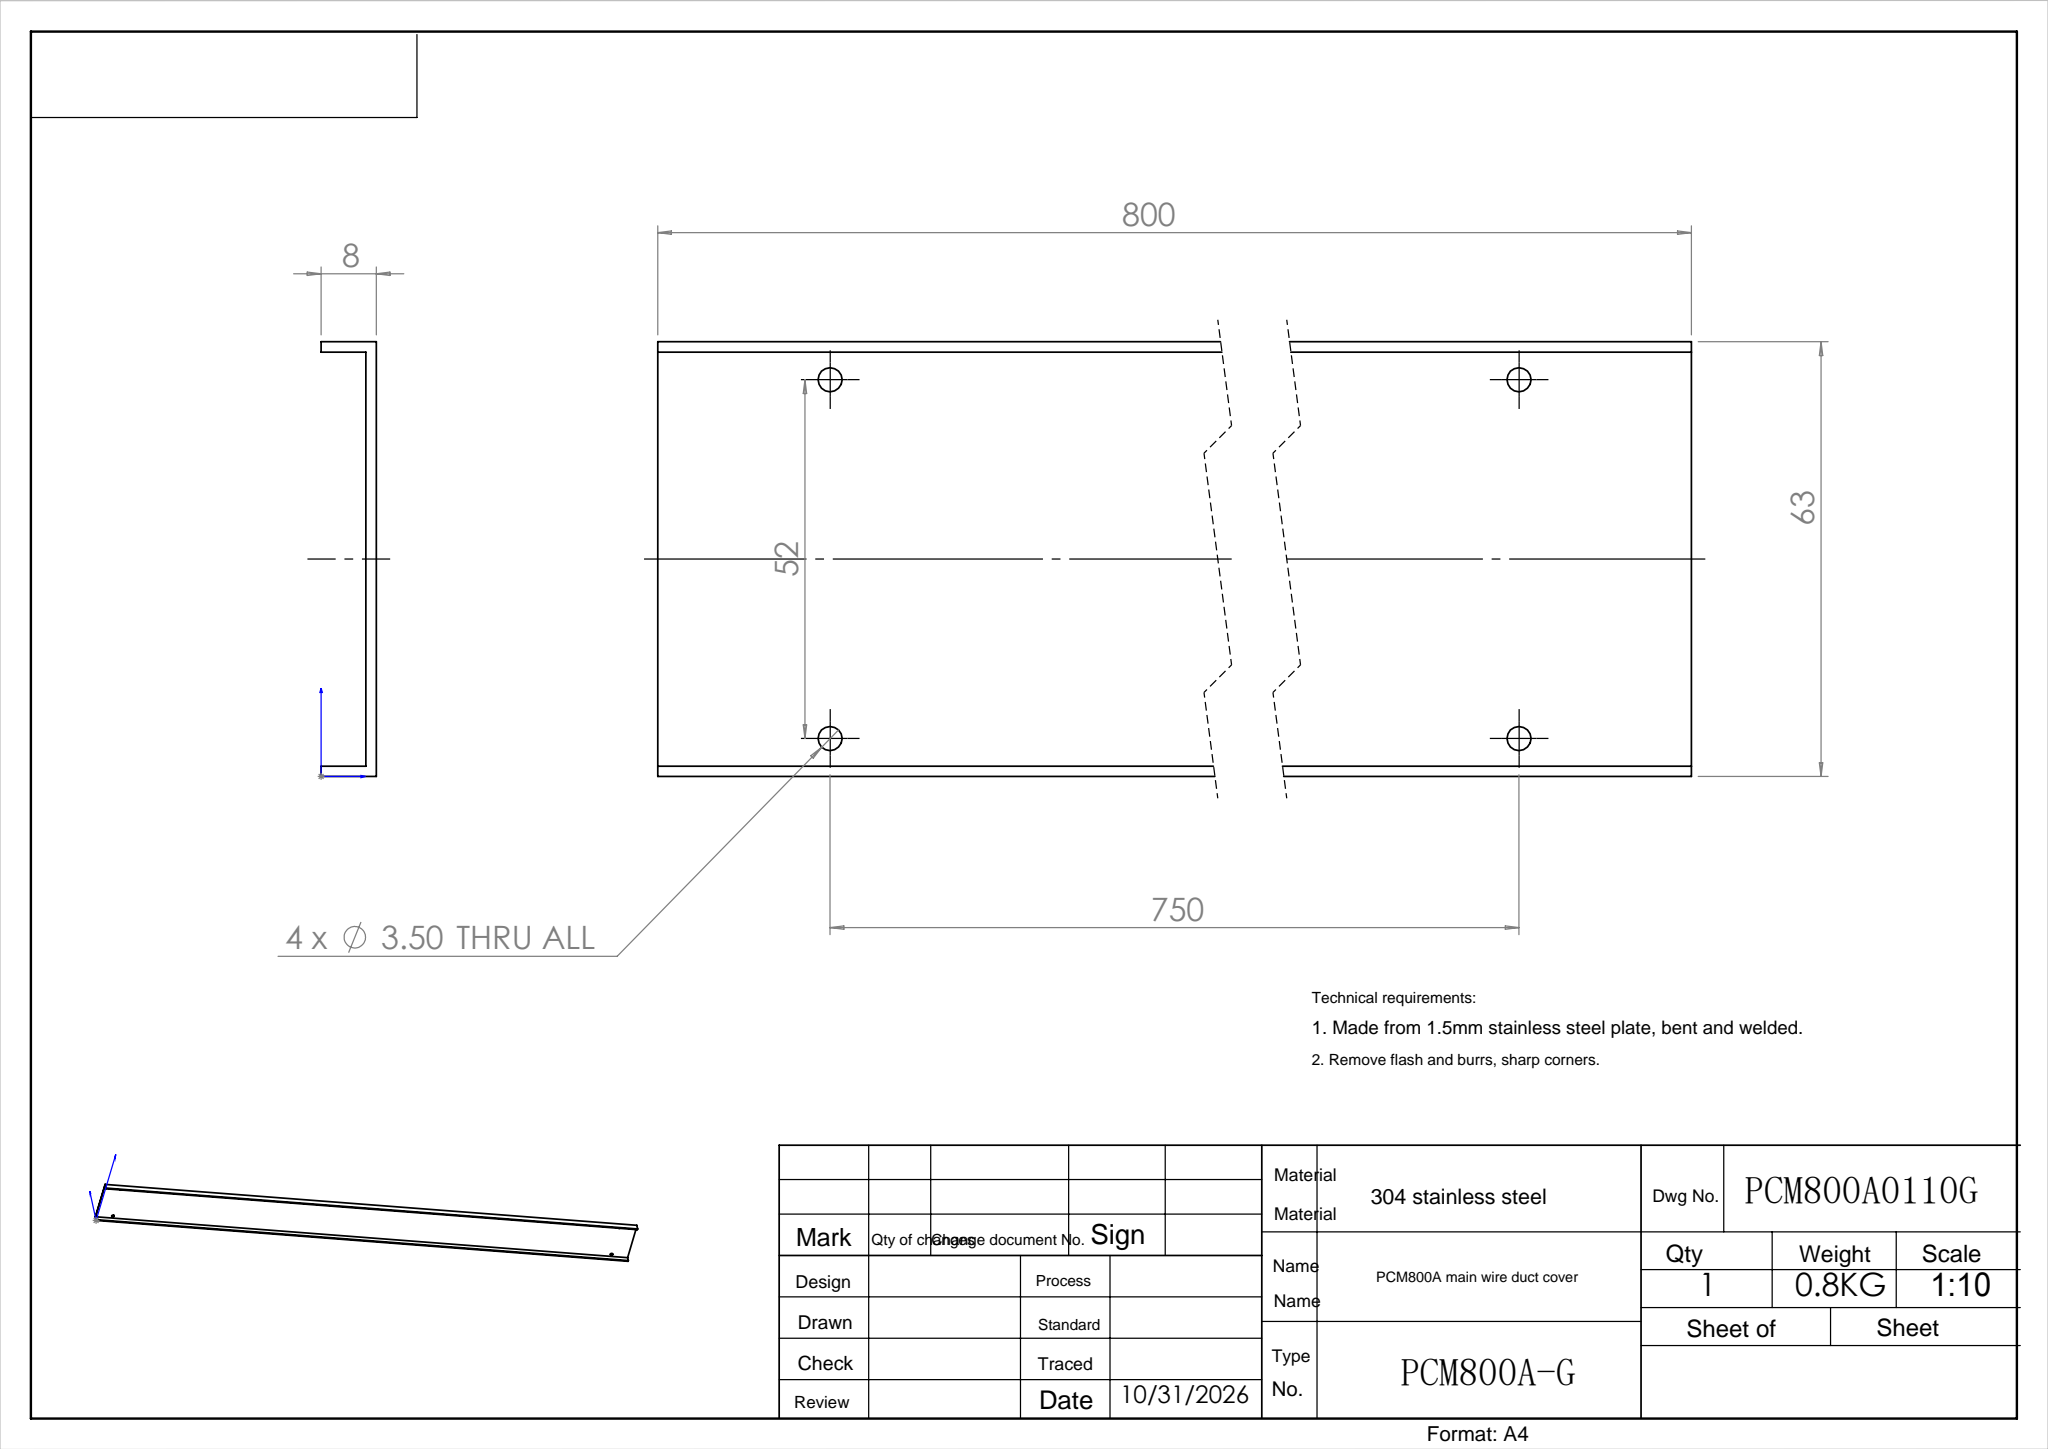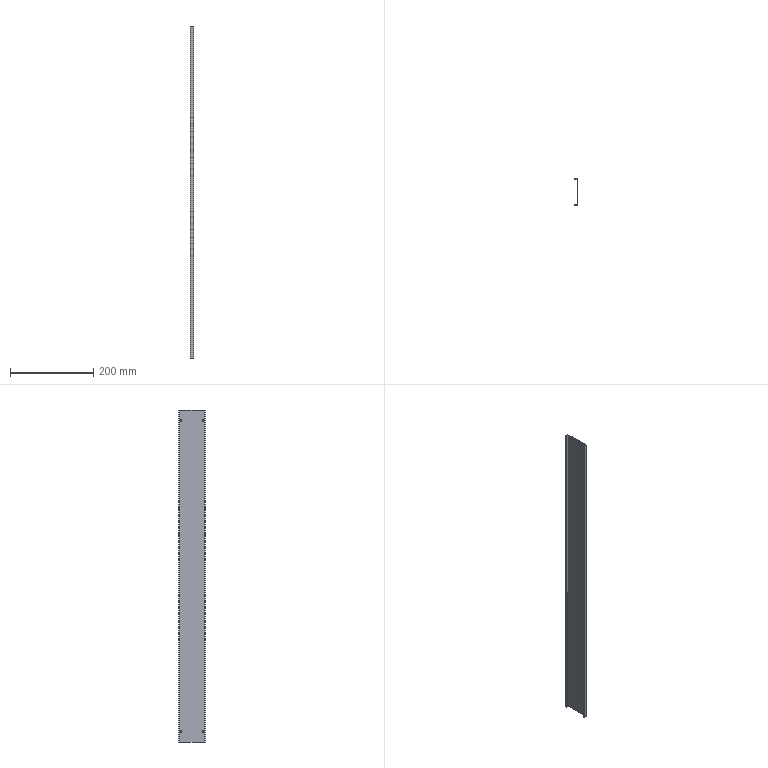Part | SolidWorks | features ExtruThin 1, HoleWzd 1, MirrorPattern 1 | 1 solid | 18 faces | box 8 x 63 x 800 mm | volume 91142 mm3 | plane 10 | cylinder 8 | commonest cylinder face diameters 3.5 x8
STEP:
#1=CARTESIAN_POINT('',(6.5,5.5,773.25));
#2=VERTEX_POINT('',#1);
#3=CARTESIAN_POINT('',(6.5,5.5,776.75));
#4=VERTEX_POINT('',#3);
#5=CARTESIAN_POINT('',(6.5,5.5,775.));
#6=DIRECTION('',(-1.,0.,0.));
#7=DIRECTION('',(0.,0.,1.));
#8=AXIS2_PLACEMENT_3D('',#5,#6,#7);
#9=CIRCLE('',#8,1.75);
#10=EDGE_CURVE('',#2,#4,#9,.T.);
#11=ORIENTED_EDGE('',*,*,#10,.T.);
#12=CARTESIAN_POINT('',(8.,5.5,776.75));
#13=VERTEX_POINT('',#12);
#14=CARTESIAN_POINT('',(8.,5.5,776.75));
#15=DIRECTION('',(1.,0.,0.));
#16=VECTOR('',#15,1000.);
#17=LINE('',#14,#16);
#18=EDGE_CURVE('',#4,#13,#17,.T.);
#19=ORIENTED_EDGE('',*,*,#18,.T.);
#20=CARTESIAN_POINT('',(8.,5.5,773.25));
#21=VERTEX_POINT('',#20);
#22=CARTESIAN_POINT('',(8.,5.5,775.));
#23=DIRECTION('',(1.,0.,0.));
#24=DIRECTION('',(0.,0.,-1.));
#25=AXIS2_PLACEMENT_3D('',#22,#23,#24);
#26=CIRCLE('',#25,1.75);
#27=EDGE_CURVE('',#13,#21,#26,.T.);
#28=ORIENTED_EDGE('',*,*,#27,.T.);
#29=CARTESIAN_POINT('',(8.,5.5,773.25));
#30=DIRECTION('',(1.,0.,0.));
#31=VECTOR('',#30,1000.);
#32=LINE('',#29,#31);
#33=EDGE_CURVE('',#2,#21,#32,.T.);
#34=ORIENTED_EDGE('',*,*,#33,.F.);
#35=EDGE_LOOP('',(#11,#19,#28,#34));
#36=FACE_OUTER_BOUND('',#35,.T.);
#37=CARTESIAN_POINT('',(8.,5.5,775.));
#38=DIRECTION('',(1.,0.,0.));
#39=DIRECTION('',(0.,0.,-1.));
#40=AXIS2_PLACEMENT_3D('',#37,#38,#39);
#41=CYLINDRICAL_SURFACE('',#40,1.75);
#42=ADVANCED_FACE('',(#36),#41,.F.);
#43=CARTESIAN_POINT('',(6.5,5.5,23.25));
#44=VERTEX_POINT('',#43);
#45=CARTESIAN_POINT('',(6.5,5.5,26.75));
#46=VERTEX_POINT('',#45);
#47=CARTESIAN_POINT('',(6.5,5.5,25.));
#48=DIRECTION('',(-1.,0.,0.));
#49=DIRECTION('',(0.,0.,1.));
#50=AXIS2_PLACEMENT_3D('',#47,#48,#49);
#51=CIRCLE('',#50,1.75);
#52=EDGE_CURVE('',#44,#46,#51,.T.);
#53=ORIENTED_EDGE('',*,*,#52,.T.);
#54=CARTESIAN_POINT('',(8.,5.5,26.75));
#55=VERTEX_POINT('',#54);
#56=CARTESIAN_POINT('',(8.,5.5,26.75));
#57=DIRECTION('',(1.,0.,0.));
#58=VECTOR('',#57,1000.);
#59=LINE('',#56,#58);
#60=EDGE_CURVE('',#46,#55,#59,.T.);
#61=ORIENTED_EDGE('',*,*,#60,.T.);
#62=CARTESIAN_POINT('',(8.,5.5,23.25));
#63=VERTEX_POINT('',#62);
#64=CARTESIAN_POINT('',(8.,5.5,25.));
#65=DIRECTION('',(1.,0.,0.));
#66=DIRECTION('',(0.,0.,-1.));
#67=AXIS2_PLACEMENT_3D('',#64,#65,#66);
#68=CIRCLE('',#67,1.75);
#69=EDGE_CURVE('',#55,#63,#68,.T.);
#70=ORIENTED_EDGE('',*,*,#69,.T.);
#71=CARTESIAN_POINT('',(8.,5.5,23.25));
#72=DIRECTION('',(1.,0.,0.));
#73=VECTOR('',#72,1000.);
#74=LINE('',#71,#73);
#75=EDGE_CURVE('',#44,#63,#74,.T.);
#76=ORIENTED_EDGE('',*,*,#75,.F.);
#77=EDGE_LOOP('',(#53,#61,#70,#76));
#78=FACE_OUTER_BOUND('',#77,.T.);
#79=CARTESIAN_POINT('',(8.,5.5,25.));
#80=DIRECTION('',(1.,0.,0.));
#81=DIRECTION('',(0.,0.,-1.));
#82=AXIS2_PLACEMENT_3D('',#79,#80,#81);
#83=CYLINDRICAL_SURFACE('',#82,1.75);
#84=ADVANCED_FACE('',(#78),#83,.F.);
#85=CARTESIAN_POINT('',(6.5,57.5,773.25));
#86=VERTEX_POINT('',#85);
#87=CARTESIAN_POINT('',(6.5,57.5,776.75));
#88=VERTEX_POINT('',#87);
#89=CARTESIAN_POINT('',(6.5,57.5,775.));
#90=DIRECTION('',(-1.,0.,0.));
#91=DIRECTION('',(0.,0.,1.));
#92=AXIS2_PLACEMENT_3D('',#89,#90,#91);
#93=CIRCLE('',#92,1.75);
#94=EDGE_CURVE('',#86,#88,#93,.T.);
#95=ORIENTED_EDGE('',*,*,#94,.T.);
#96=CARTESIAN_POINT('',(8.,57.5,776.75));
#97=VERTEX_POINT('',#96);
#98=CARTESIAN_POINT('',(8.,57.5,776.75));
#99=DIRECTION('',(1.,0.,0.));
#100=VECTOR('',#99,1000.);
#101=LINE('',#98,#100);
#102=EDGE_CURVE('',#88,#97,#101,.T.);
#103=ORIENTED_EDGE('',*,*,#102,.T.);
#104=CARTESIAN_POINT('',(8.,57.5,773.25));
#105=VERTEX_POINT('',#104);
#106=CARTESIAN_POINT('',(8.,57.5,775.));
#107=DIRECTION('',(1.,0.,0.));
#108=DIRECTION('',(0.,0.,-1.));
#109=AXIS2_PLACEMENT_3D('',#106,#107,#108);
#110=CIRCLE('',#109,1.75);
#111=EDGE_CURVE('',#97,#105,#110,.T.);
#112=ORIENTED_EDGE('',*,*,#111,.T.);
#113=CARTESIAN_POINT('',(8.,57.5,773.25));
#114=DIRECTION('',(1.,0.,0.));
#115=VECTOR('',#114,1000.);
#116=LINE('',#113,#115);
#117=EDGE_CURVE('',#86,#105,#116,.T.);
#118=ORIENTED_EDGE('',*,*,#117,.F.);
#119=EDGE_LOOP('',(#95,#103,#112,#118));
#120=FACE_OUTER_BOUND('',#119,.T.);
#121=CARTESIAN_POINT('',(8.,57.5,775.));
#122=DIRECTION('',(1.,0.,0.));
#123=DIRECTION('',(0.,0.,-1.));
#124=AXIS2_PLACEMENT_3D('',#121,#122,#123);
#125=CYLINDRICAL_SURFACE('',#124,1.75);
#126=ADVANCED_FACE('',(#120),#125,.F.);
#127=CARTESIAN_POINT('',(6.5,57.5,23.25));
#128=VERTEX_POINT('',#127);
#129=CARTESIAN_POINT('',(6.5,57.5,26.75));
#130=VERTEX_POINT('',#129);
#131=CARTESIAN_POINT('',(6.5,57.5,25.));
#132=DIRECTION('',(-1.,0.,0.));
#133=DIRECTION('',(0.,0.,1.));
#134=AXIS2_PLACEMENT_3D('',#131,#132,#133);
#135=CIRCLE('',#134,1.75);
#136=EDGE_CURVE('',#128,#130,#135,.T.);
#137=ORIENTED_EDGE('',*,*,#136,.T.);
#138=CARTESIAN_POINT('',(8.,57.5,26.75));
#139=VERTEX_POINT('',#138);
#140=CARTESIAN_POINT('',(8.,57.5,26.75));
#141=DIRECTION('',(1.,0.,0.));
#142=VECTOR('',#141,1000.);
#143=LINE('',#140,#142);
#144=EDGE_CURVE('',#130,#139,#143,.T.);
#145=ORIENTED_EDGE('',*,*,#144,.T.);
#146=CARTESIAN_POINT('',(8.,57.5,23.25));
#147=VERTEX_POINT('',#146);
#148=CARTESIAN_POINT('',(8.,57.5,25.));
#149=DIRECTION('',(1.,0.,0.));
#150=DIRECTION('',(0.,0.,-1.));
#151=AXIS2_PLACEMENT_3D('',#148,#149,#150);
#152=CIRCLE('',#151,1.75);
#153=EDGE_CURVE('',#139,#147,#152,.T.);
#154=ORIENTED_EDGE('',*,*,#153,.T.);
#155=CARTESIAN_POINT('',(8.,57.5,23.25));
#156=DIRECTION('',(1.,0.,0.));
#157=VECTOR('',#156,1000.);
#158=LINE('',#155,#157);
#159=EDGE_CURVE('',#128,#147,#158,.T.);
#160=ORIENTED_EDGE('',*,*,#159,.F.);
#161=EDGE_LOOP('',(#137,#145,#154,#160));
#162=FACE_OUTER_BOUND('',#161,.T.);
#163=CARTESIAN_POINT('',(8.,57.5,25.));
#164=DIRECTION('',(1.,0.,0.));
#165=DIRECTION('',(0.,0.,-1.));
#166=AXIS2_PLACEMENT_3D('',#163,#164,#165);
#167=CYLINDRICAL_SURFACE('',#166,1.75);
#168=ADVANCED_FACE('',(#162),#167,.F.);
#169=CARTESIAN_POINT('',(8.,63.,0.));
#170=VERTEX_POINT('',#169);
#171=CARTESIAN_POINT('',(0.,63.,0.));
#172=VERTEX_POINT('',#171);
#173=CARTESIAN_POINT('',(8.,63.,0.));
#174=DIRECTION('',(-1.,0.,0.));
#175=VECTOR('',#174,1000.);
#176=LINE('',#173,#175);
#177=EDGE_CURVE('',#170,#172,#176,.T.);
#178=ORIENTED_EDGE('',*,*,#177,.T.);
#179=CARTESIAN_POINT('',(0.,63.,800.));
#180=VERTEX_POINT('',#179);
#181=CARTESIAN_POINT('',(0.,63.,800.));
#182=DIRECTION('',(0.,0.,-1.));
#183=VECTOR('',#182,1000.);
#184=LINE('',#181,#183);
#185=EDGE_CURVE('',#180,#172,#184,.T.);
#186=ORIENTED_EDGE('',*,*,#185,.F.);
#187=CARTESIAN_POINT('',(8.,63.,800.));
#188=VERTEX_POINT('',#187);
#189=CARTESIAN_POINT('',(8.,63.,800.));
#190=DIRECTION('',(-1.,0.,0.));
#191=VECTOR('',#190,1000.);
#192=LINE('',#189,#191);
#193=EDGE_CURVE('',#188,#180,#192,.T.);
#194=ORIENTED_EDGE('',*,*,#193,.F.);
#195=CARTESIAN_POINT('',(8.,63.,800.));
#196=DIRECTION('',(0.,0.,-1.));
#197=VECTOR('',#196,1000.);
#198=LINE('',#195,#197);
#199=EDGE_CURVE('',#188,#170,#198,.T.);
#200=ORIENTED_EDGE('',*,*,#199,.T.);
#201=EDGE_LOOP('',(#178,#186,#194,#200));
#202=FACE_OUTER_BOUND('',#201,.T.);
#203=CARTESIAN_POINT('',(8.,63.,800.));
#204=DIRECTION('',(0.,-1.,0.));
#205=DIRECTION('',(0.,0.,-1.));
#206=AXIS2_PLACEMENT_3D('',#203,#204,#205);
#207=PLANE('',#206);
#208=ADVANCED_FACE('',(#202),#207,.F.);
#209=CARTESIAN_POINT('',(0.,61.5,0.));
#210=VERTEX_POINT('',#209);
#211=CARTESIAN_POINT('',(0.,61.5,0.));
#212=DIRECTION('',(0.,1.,0.));
#213=VECTOR('',#212,1000.);
#214=LINE('',#211,#213);
#215=EDGE_CURVE('',#210,#172,#214,.T.);
#216=ORIENTED_EDGE('',*,*,#215,.F.);
#217=CARTESIAN_POINT('',(0.,61.5,800.));
#218=VERTEX_POINT('',#217);
#219=CARTESIAN_POINT('',(0.,61.5,800.));
#220=DIRECTION('',(0.,0.,-1.));
#221=VECTOR('',#220,1000.);
#222=LINE('',#219,#221);
#223=EDGE_CURVE('',#218,#210,#222,.T.);
#224=ORIENTED_EDGE('',*,*,#223,.F.);
#225=CARTESIAN_POINT('',(0.,61.5,800.));
#226=DIRECTION('',(0.,1.,0.));
#227=VECTOR('',#226,1000.);
#228=LINE('',#225,#227);
#229=EDGE_CURVE('',#218,#180,#228,.T.);
#230=ORIENTED_EDGE('',*,*,#229,.T.);
#231=ORIENTED_EDGE('',*,*,#185,.T.);
#232=EDGE_LOOP('',(#216,#224,#230,#231));
#233=FACE_OUTER_BOUND('',#232,.T.);
#234=CARTESIAN_POINT('',(0.,61.5,800.));
#235=DIRECTION('',(-1.,0.,0.));
#236=DIRECTION('',(0.,0.,1.));
#237=AXIS2_PLACEMENT_3D('',#234,#235,#236);
#238=PLANE('',#237);
#239=ADVANCED_FACE('',(#233),#238,.T.);
#240=CARTESIAN_POINT('',(6.5,61.5,0.));
#241=VERTEX_POINT('',#240);
#242=CARTESIAN_POINT('',(8.,61.5,0.));
#243=DIRECTION('',(-1.,0.,0.));
#244=VECTOR('',#243,1000.);
#245=LINE('',#242,#244);
#246=EDGE_CURVE('',#241,#210,#245,.T.);
#247=ORIENTED_EDGE('',*,*,#246,.F.);
#248=CARTESIAN_POINT('',(6.5,61.5,800.));
#249=VERTEX_POINT('',#248);
#250=CARTESIAN_POINT('',(6.5,61.5,800.));
#251=DIRECTION('',(0.,0.,-1.));
#252=VECTOR('',#251,1000.);
#253=LINE('',#250,#252);
#254=EDGE_CURVE('',#249,#241,#253,.T.);
#255=ORIENTED_EDGE('',*,*,#254,.F.);
#256=CARTESIAN_POINT('',(8.,61.5,800.));
#257=DIRECTION('',(-1.,0.,0.));
#258=VECTOR('',#257,1000.);
#259=LINE('',#256,#258);
#260=EDGE_CURVE('',#249,#218,#259,.T.);
#261=ORIENTED_EDGE('',*,*,#260,.T.);
#262=ORIENTED_EDGE('',*,*,#223,.T.);
#263=EDGE_LOOP('',(#247,#255,#261,#262));
#264=FACE_OUTER_BOUND('',#263,.T.);
#265=CARTESIAN_POINT('',(8.,61.5,800.));
#266=DIRECTION('',(0.,-1.,0.));
#267=DIRECTION('',(0.,0.,-1.));
#268=AXIS2_PLACEMENT_3D('',#265,#266,#267);
#269=PLANE('',#268);
#270=ADVANCED_FACE('',(#264),#269,.T.);
#271=ORIENTED_EDGE('',*,*,#10,.F.);
#272=CARTESIAN_POINT('',(6.5,5.5,775.));
#273=DIRECTION('',(-1.,0.,0.));
#274=DIRECTION('',(0.,0.,1.));
#275=AXIS2_PLACEMENT_3D('',#272,#273,#274);
#276=CIRCLE('',#275,1.75);
#277=EDGE_CURVE('',#4,#2,#276,.T.);
#278=ORIENTED_EDGE('',*,*,#277,.F.);
#279=EDGE_LOOP('',(#271,#278));
#280=FACE_BOUND('',#279,.T.);
#281=ORIENTED_EDGE('',*,*,#52,.F.);
#282=CARTESIAN_POINT('',(6.5,5.5,25.));
#283=DIRECTION('',(-1.,0.,0.));
#284=DIRECTION('',(0.,0.,1.));
#285=AXIS2_PLACEMENT_3D('',#282,#283,#284);
#286=CIRCLE('',#285,1.75);
#287=EDGE_CURVE('',#46,#44,#286,.T.);
#288=ORIENTED_EDGE('',*,*,#287,.F.);
#289=EDGE_LOOP('',(#281,#288));
#290=FACE_BOUND('',#289,.T.);
#291=ORIENTED_EDGE('',*,*,#94,.F.);
#292=CARTESIAN_POINT('',(6.5,57.5,775.));
#293=DIRECTION('',(-1.,0.,0.));
#294=DIRECTION('',(0.,0.,1.));
#295=AXIS2_PLACEMENT_3D('',#292,#293,#294);
#296=CIRCLE('',#295,1.75);
#297=EDGE_CURVE('',#88,#86,#296,.T.);
#298=ORIENTED_EDGE('',*,*,#297,.F.);
#299=EDGE_LOOP('',(#291,#298));
#300=FACE_BOUND('',#299,.T.);
#301=ORIENTED_EDGE('',*,*,#136,.F.);
#302=CARTESIAN_POINT('',(6.5,57.5,25.));
#303=DIRECTION('',(-1.,0.,0.));
#304=DIRECTION('',(0.,0.,1.));
#305=AXIS2_PLACEMENT_3D('',#302,#303,#304);
#306=CIRCLE('',#305,1.75);
#307=EDGE_CURVE('',#130,#128,#306,.T.);
#308=ORIENTED_EDGE('',*,*,#307,.F.);
#309=EDGE_LOOP('',(#301,#308));
#310=FACE_BOUND('',#309,.T.);
#311=CARTESIAN_POINT('',(6.5,1.5,0.));
#312=VERTEX_POINT('',#311);
#313=CARTESIAN_POINT('',(6.5,0.,0.));
#314=DIRECTION('',(0.,1.,0.));
#315=VECTOR('',#314,1000.);
#316=LINE('',#313,#315);
#317=EDGE_CURVE('',#312,#241,#316,.T.);
#318=ORIENTED_EDGE('',*,*,#317,.F.);
#319=CARTESIAN_POINT('',(6.5,1.5,800.));
#320=VERTEX_POINT('',#319);
#321=CARTESIAN_POINT('',(6.5,1.5,800.));
#322=DIRECTION('',(0.,0.,-1.));
#323=VECTOR('',#322,1000.);
#324=LINE('',#321,#323);
#325=EDGE_CURVE('',#320,#312,#324,.T.);
#326=ORIENTED_EDGE('',*,*,#325,.F.);
#327=CARTESIAN_POINT('',(6.5,0.,800.));
#328=DIRECTION('',(0.,1.,0.));
#329=VECTOR('',#328,1000.);
#330=LINE('',#327,#329);
#331=EDGE_CURVE('',#320,#249,#330,.T.);
#332=ORIENTED_EDGE('',*,*,#331,.T.);
#333=ORIENTED_EDGE('',*,*,#254,.T.);
#334=EDGE_LOOP('',(#318,#326,#332,#333));
#335=FACE_OUTER_BOUND('',#334,.T.);
#336=CARTESIAN_POINT('',(6.5,0.,800.));
#337=DIRECTION('',(-1.,0.,0.));
#338=DIRECTION('',(0.,0.,1.));
#339=AXIS2_PLACEMENT_3D('',#336,#337,#338);
#340=PLANE('',#339);
#341=ADVANCED_FACE('',(#280,#290,#300,#310,#335),#340,.T.);
#342=CARTESIAN_POINT('',(0.,1.5,0.));
#343=VERTEX_POINT('',#342);
#344=CARTESIAN_POINT('',(0.,1.5,0.));
#345=DIRECTION('',(1.,0.,0.));
#346=VECTOR('',#345,1000.);
#347=LINE('',#344,#346);
#348=EDGE_CURVE('',#343,#312,#347,.T.);
#349=ORIENTED_EDGE('',*,*,#348,.F.);
#350=CARTESIAN_POINT('',(0.,1.5,800.));
#351=VERTEX_POINT('',#350);
#352=CARTESIAN_POINT('',(0.,1.5,800.));
#353=DIRECTION('',(0.,0.,-1.));
#354=VECTOR('',#353,1000.);
#355=LINE('',#352,#354);
#356=EDGE_CURVE('',#351,#343,#355,.T.);
#357=ORIENTED_EDGE('',*,*,#356,.F.);
#358=CARTESIAN_POINT('',(0.,1.5,800.));
#359=DIRECTION('',(1.,0.,0.));
#360=VECTOR('',#359,1000.);
#361=LINE('',#358,#360);
#362=EDGE_CURVE('',#351,#320,#361,.T.);
#363=ORIENTED_EDGE('',*,*,#362,.T.);
#364=ORIENTED_EDGE('',*,*,#325,.T.);
#365=EDGE_LOOP('',(#349,#357,#363,#364));
#366=FACE_OUTER_BOUND('',#365,.T.);
#367=CARTESIAN_POINT('',(0.,1.5,800.));
#368=DIRECTION('',(0.,1.,0.));
#369=DIRECTION('',(0.,0.,1.));
#370=AXIS2_PLACEMENT_3D('',#367,#368,#369);
#371=PLANE('',#370);
#372=ADVANCED_FACE('',(#366),#371,.T.);
#373=CARTESIAN_POINT('',(0.,0.,0.));
#374=VERTEX_POINT('',#373);
#375=CARTESIAN_POINT('',(0.,0.,0.));
#376=DIRECTION('',(0.,1.,0.));
#377=VECTOR('',#376,1000.);
#378=LINE('',#375,#377);
#379=EDGE_CURVE('',#374,#343,#378,.T.);
#380=ORIENTED_EDGE('',*,*,#379,.F.);
#381=CARTESIAN_POINT('',(0.,0.,800.));
#382=VERTEX_POINT('',#381);
#383=CARTESIAN_POINT('',(0.,0.,800.));
#384=DIRECTION('',(0.,0.,-1.));
#385=VECTOR('',#384,1000.);
#386=LINE('',#383,#385);
#387=EDGE_CURVE('',#382,#374,#386,.T.);
#388=ORIENTED_EDGE('',*,*,#387,.F.);
#389=CARTESIAN_POINT('',(0.,0.,800.));
#390=DIRECTION('',(0.,1.,0.));
#391=VECTOR('',#390,1000.);
#392=LINE('',#389,#391);
#393=EDGE_CURVE('',#382,#351,#392,.T.);
#394=ORIENTED_EDGE('',*,*,#393,.T.);
#395=ORIENTED_EDGE('',*,*,#356,.T.);
#396=EDGE_LOOP('',(#380,#388,#394,#395));
#397=FACE_OUTER_BOUND('',#396,.T.);
#398=CARTESIAN_POINT('',(0.,0.,800.));
#399=DIRECTION('',(-1.,0.,0.));
#400=DIRECTION('',(0.,0.,1.));
#401=AXIS2_PLACEMENT_3D('',#398,#399,#400);
#402=PLANE('',#401);
#403=ADVANCED_FACE('',(#397),#402,.T.);
#404=CARTESIAN_POINT('',(8.,0.,0.));
#405=VERTEX_POINT('',#404);
#406=CARTESIAN_POINT('',(0.,0.,0.));
#407=DIRECTION('',(1.,0.,0.));
#408=VECTOR('',#407,1000.);
#409=LINE('',#406,#408);
#410=EDGE_CURVE('',#374,#405,#409,.T.);
#411=ORIENTED_EDGE('',*,*,#410,.T.);
#412=CARTESIAN_POINT('',(8.,0.,800.));
#413=VERTEX_POINT('',#412);
#414=CARTESIAN_POINT('',(8.,0.,800.));
#415=DIRECTION('',(0.,0.,-1.));
#416=VECTOR('',#415,1000.);
#417=LINE('',#414,#416);
#418=EDGE_CURVE('',#413,#405,#417,.T.);
#419=ORIENTED_EDGE('',*,*,#418,.F.);
#420=CARTESIAN_POINT('',(0.,0.,800.));
#421=DIRECTION('',(1.,0.,0.));
#422=VECTOR('',#421,1000.);
#423=LINE('',#420,#422);
#424=EDGE_CURVE('',#382,#413,#423,.T.);
#425=ORIENTED_EDGE('',*,*,#424,.F.);
#426=ORIENTED_EDGE('',*,*,#387,.T.);
#427=EDGE_LOOP('',(#411,#419,#425,#426));
#428=FACE_OUTER_BOUND('',#427,.T.);
#429=CARTESIAN_POINT('',(0.,0.,800.));
#430=DIRECTION('',(0.,1.,0.));
#431=DIRECTION('',(0.,0.,1.));
#432=AXIS2_PLACEMENT_3D('',#429,#430,#431);
#433=PLANE('',#432);
#434=ADVANCED_FACE('',(#428),#433,.F.);
#435=CARTESIAN_POINT('',(8.,5.5,775.));
#436=DIRECTION('',(1.,0.,0.));
#437=DIRECTION('',(0.,0.,-1.));
#438=AXIS2_PLACEMENT_3D('',#435,#436,#437);
#439=CIRCLE('',#438,1.75);
#440=EDGE_CURVE('',#21,#13,#439,.T.);
#441=ORIENTED_EDGE('',*,*,#440,.F.);
#442=ORIENTED_EDGE('',*,*,#27,.F.);
#443=EDGE_LOOP('',(#441,#442));
#444=FACE_BOUND('',#443,.T.);
#445=CARTESIAN_POINT('',(8.,5.5,25.));
#446=DIRECTION('',(1.,0.,0.));
#447=DIRECTION('',(0.,0.,-1.));
#448=AXIS2_PLACEMENT_3D('',#445,#446,#447);
#449=CIRCLE('',#448,1.75);
#450=EDGE_CURVE('',#63,#55,#449,.T.);
#451=ORIENTED_EDGE('',*,*,#450,.F.);
#452=ORIENTED_EDGE('',*,*,#69,.F.);
#453=EDGE_LOOP('',(#451,#452));
#454=FACE_BOUND('',#453,.T.);
#455=CARTESIAN_POINT('',(8.,57.5,775.));
#456=DIRECTION('',(1.,0.,0.));
#457=DIRECTION('',(0.,0.,-1.));
#458=AXIS2_PLACEMENT_3D('',#455,#456,#457);
#459=CIRCLE('',#458,1.75);
#460=EDGE_CURVE('',#105,#97,#459,.T.);
#461=ORIENTED_EDGE('',*,*,#460,.F.);
#462=ORIENTED_EDGE('',*,*,#111,.F.);
#463=EDGE_LOOP('',(#461,#462));
#464=FACE_BOUND('',#463,.T.);
#465=CARTESIAN_POINT('',(8.,57.5,25.));
#466=DIRECTION('',(1.,0.,0.));
#467=DIRECTION('',(0.,0.,-1.));
#468=AXIS2_PLACEMENT_3D('',#465,#466,#467);
#469=CIRCLE('',#468,1.75);
#470=EDGE_CURVE('',#147,#139,#469,.T.);
#471=ORIENTED_EDGE('',*,*,#470,.F.);
#472=ORIENTED_EDGE('',*,*,#153,.F.);
#473=EDGE_LOOP('',(#471,#472));
#474=FACE_BOUND('',#473,.T.);
#475=CARTESIAN_POINT('',(8.,0.,0.));
#476=DIRECTION('',(0.,1.,0.));
#477=VECTOR('',#476,1000.);
#478=LINE('',#475,#477);
#479=EDGE_CURVE('',#405,#170,#478,.T.);
#480=ORIENTED_EDGE('',*,*,#479,.T.);
#481=ORIENTED_EDGE('',*,*,#199,.F.);
#482=CARTESIAN_POINT('',(8.,0.,800.));
#483=DIRECTION('',(0.,1.,0.));
#484=VECTOR('',#483,1000.);
#485=LINE('',#482,#484);
#486=EDGE_CURVE('',#413,#188,#485,.T.);
#487=ORIENTED_EDGE('',*,*,#486,.F.);
#488=ORIENTED_EDGE('',*,*,#418,.T.);
#489=EDGE_LOOP('',(#480,#481,#487,#488));
#490=FACE_OUTER_BOUND('',#489,.T.);
#491=CARTESIAN_POINT('',(8.,0.,800.));
#492=DIRECTION('',(-1.,0.,0.));
#493=DIRECTION('',(0.,0.,1.));
#494=AXIS2_PLACEMENT_3D('',#491,#492,#493);
#495=PLANE('',#494);
#496=ADVANCED_FACE('',(#444,#454,#464,#474,#490),#495,.F.);
#497=ORIENTED_EDGE('',*,*,#193,.T.);
#498=ORIENTED_EDGE('',*,*,#229,.F.);
#499=ORIENTED_EDGE('',*,*,#260,.F.);
#500=ORIENTED_EDGE('',*,*,#331,.F.);
#501=ORIENTED_EDGE('',*,*,#362,.F.);
#502=ORIENTED_EDGE('',*,*,#393,.F.);
#503=ORIENTED_EDGE('',*,*,#424,.T.);
#504=ORIENTED_EDGE('',*,*,#486,.T.);
#505=EDGE_LOOP('',(#497,#498,#499,#500,#501,#502,#503,#504));
#506=FACE_OUTER_BOUND('',#505,.T.);
#507=CARTESIAN_POINT('',(0.,63.,800.));
#508=DIRECTION('',(0.,0.,-1.));
#509=DIRECTION('',(-1.,0.,0.));
#510=AXIS2_PLACEMENT_3D('',#507,#508,#509);
#511=PLANE('',#510);
#512=ADVANCED_FACE('',(#506),#511,.F.);
#513=ORIENTED_EDGE('',*,*,#177,.F.);
#514=ORIENTED_EDGE('',*,*,#479,.F.);
#515=ORIENTED_EDGE('',*,*,#410,.F.);
#516=ORIENTED_EDGE('',*,*,#379,.T.);
#517=ORIENTED_EDGE('',*,*,#348,.T.);
#518=ORIENTED_EDGE('',*,*,#317,.T.);
#519=ORIENTED_EDGE('',*,*,#246,.T.);
#520=ORIENTED_EDGE('',*,*,#215,.T.);
#521=EDGE_LOOP('',(#513,#514,#515,#516,#517,#518,#519,#520));
#522=FACE_OUTER_BOUND('',#521,.T.);
#523=CARTESIAN_POINT('',(0.,63.,0.));
#524=DIRECTION('',(0.,0.,-1.));
#525=DIRECTION('',(-1.,0.,0.));
#526=AXIS2_PLACEMENT_3D('',#523,#524,#525);
#527=PLANE('',#526);
#528=ADVANCED_FACE('',(#522),#527,.T.);
#529=ORIENTED_EDGE('',*,*,#144,.F.);
#530=ORIENTED_EDGE('',*,*,#307,.T.);
#531=ORIENTED_EDGE('',*,*,#159,.T.);
#532=ORIENTED_EDGE('',*,*,#470,.T.);
#533=EDGE_LOOP('',(#529,#530,#531,#532));
#534=FACE_OUTER_BOUND('',#533,.T.);
#535=CARTESIAN_POINT('',(8.,57.5,25.));
#536=DIRECTION('',(1.,0.,0.));
#537=DIRECTION('',(0.,0.,-1.));
#538=AXIS2_PLACEMENT_3D('',#535,#536,#537);
#539=CYLINDRICAL_SURFACE('',#538,1.75);
#540=ADVANCED_FACE('',(#534),#539,.F.);
#541=ORIENTED_EDGE('',*,*,#102,.F.);
#542=ORIENTED_EDGE('',*,*,#297,.T.);
#543=ORIENTED_EDGE('',*,*,#117,.T.);
#544=ORIENTED_EDGE('',*,*,#460,.T.);
#545=EDGE_LOOP('',(#541,#542,#543,#544));
#546=FACE_OUTER_BOUND('',#545,.T.);
#547=CARTESIAN_POINT('',(8.,57.5,775.));
#548=DIRECTION('',(1.,0.,0.));
#549=DIRECTION('',(0.,0.,-1.));
#550=AXIS2_PLACEMENT_3D('',#547,#548,#549);
#551=CYLINDRICAL_SURFACE('',#550,1.75);
#552=ADVANCED_FACE('',(#546),#551,.F.);
#553=ORIENTED_EDGE('',*,*,#60,.F.);
#554=ORIENTED_EDGE('',*,*,#287,.T.);
#555=ORIENTED_EDGE('',*,*,#75,.T.);
#556=ORIENTED_EDGE('',*,*,#450,.T.);
#557=EDGE_LOOP('',(#553,#554,#555,#556));
#558=FACE_OUTER_BOUND('',#557,.T.);
#559=CARTESIAN_POINT('',(8.,5.5,25.));
#560=DIRECTION('',(1.,0.,0.));
#561=DIRECTION('',(0.,0.,-1.));
#562=AXIS2_PLACEMENT_3D('',#559,#560,#561);
#563=CYLINDRICAL_SURFACE('',#562,1.75);
#564=ADVANCED_FACE('',(#558),#563,.F.);
#565=ORIENTED_EDGE('',*,*,#18,.F.);
#566=ORIENTED_EDGE('',*,*,#277,.T.);
#567=ORIENTED_EDGE('',*,*,#33,.T.);
#568=ORIENTED_EDGE('',*,*,#440,.T.);
#569=EDGE_LOOP('',(#565,#566,#567,#568));
#570=FACE_OUTER_BOUND('',#569,.T.);
#571=CARTESIAN_POINT('',(8.,5.5,775.));
#572=DIRECTION('',(1.,0.,0.));
#573=DIRECTION('',(0.,0.,-1.));
#574=AXIS2_PLACEMENT_3D('',#571,#572,#573);
#575=CYLINDRICAL_SURFACE('',#574,1.75);
#576=ADVANCED_FACE('',(#570),#575,.F.);
#577=CLOSED_SHELL('',(#42,#84,#126,#168,#208,#239,#270,#341,#372,#403,#434,#496,#512,#528,#540,#552,#564,#576));
#578=MANIFOLD_SOLID_BREP('',#577);
#579=CARTESIAN_POINT('',(0.,0.,0.));
#580=DIRECTION('',(0.,0.,1.));
#581=DIRECTION('',(1.,0.,0.));
#582=AXIS2_PLACEMENT_3D('',#579,#580,#581);
#583=(LENGTH_UNIT()NAMED_UNIT(*)SI_UNIT(.MILLI.,.METRE.));
#584=UNCERTAINTY_MEASURE_WITH_UNIT(LENGTH_MEASURE(0.00001),#583,'','');
#585=(NAMED_UNIT(*)PLANE_ANGLE_UNIT()SI_UNIT($,.RADIAN.));
#586=(NAMED_UNIT(*)SI_UNIT($,.STERADIAN.)SOLID_ANGLE_UNIT());
#587=(GEOMETRIC_REPRESENTATION_CONTEXT(3)GLOBAL_UNCERTAINTY_ASSIGNED_CONTEXT((#584))GLOBAL_UNIT_ASSIGNED_CONTEXT((#583,#585,#586))REPRESENTATION_CONTEXT('',''));
#588=ADVANCED_BREP_SHAPE_REPRESENTATION('',(#578,#582),#587);